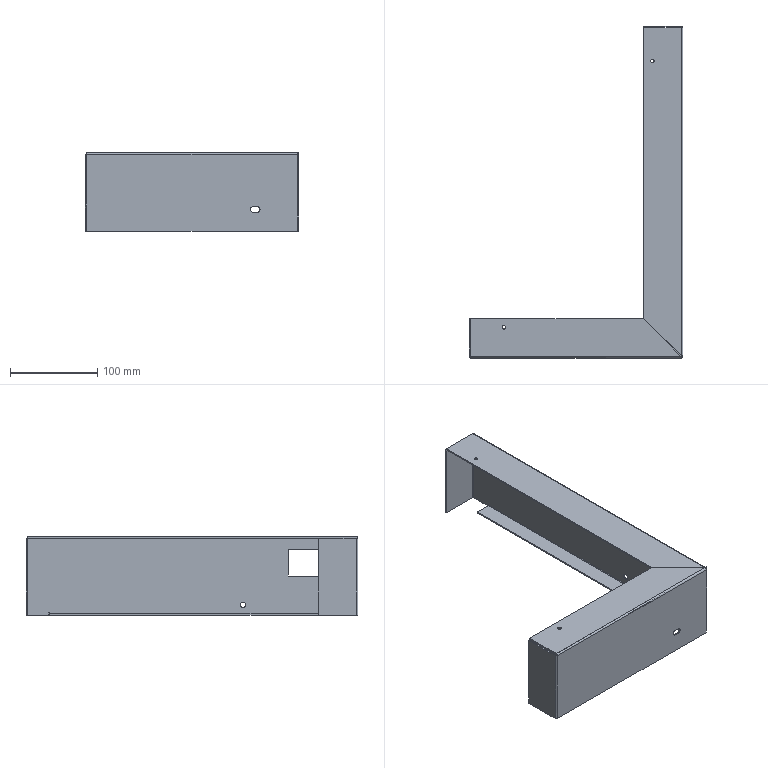Part | SolidWorks | features ICE 5, EdgeFlange 1, FlatPattern 1, SMBaseFlange 1, SMMiteredFlange 1, SheetMetal 1 | 1 solid | 76 faces | box 245 x 380 x 90 mm | volume 139211 mm3 | plane 50 | cylinder 20 | spline 6 | commonest cylinder face diameters 4 x10 1 x6 6 x2 6.4 x2